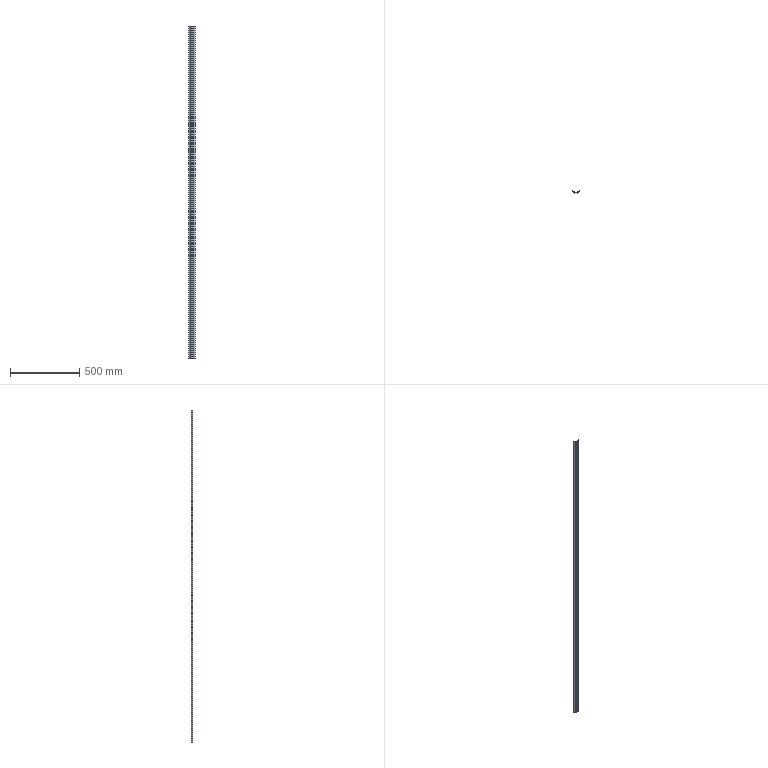Part | SolidWorks | features Extrusion 1 | 1 solid | 32 faces | box 46.782 x 13.535 x 2390 mm | volume 191944 mm3 | plane 25 | cylinder 7 | commonest cylinder face diameters 67.994 x4 0.2 x2 65.594 x1
STEP:
#1=CARTESIAN_POINT('',(-11.25,9.786,-1195.));
#2=VERTEX_POINT('',#1);
#3=CARTESIAN_POINT('',(-11.25,5.783,-1195.));
#4=VERTEX_POINT('',#3);
#5=CARTESIAN_POINT('',(-11.25,9.786,-1195.));
#6=DIRECTION('',(0.,-1.,0.));
#7=VECTOR('',#6,1000.);
#8=LINE('',#5,#7);
#9=EDGE_CURVE('',#2,#4,#8,.T.);
#10=ORIENTED_EDGE('',*,*,#9,.T.);
#11=CARTESIAN_POINT('',(-11.25,5.783,1195.));
#12=VERTEX_POINT('',#11);
#13=CARTESIAN_POINT('',(-11.25,5.783,1195.));
#14=DIRECTION('',(0.,0.,-1.));
#15=VECTOR('',#14,1000.);
#16=LINE('',#13,#15);
#17=EDGE_CURVE('',#12,#4,#16,.T.);
#18=ORIENTED_EDGE('',*,*,#17,.F.);
#19=CARTESIAN_POINT('',(-11.25,9.786,1195.));
#20=VERTEX_POINT('',#19);
#21=CARTESIAN_POINT('',(-11.25,9.786,1195.));
#22=DIRECTION('',(0.,-1.,0.));
#23=VECTOR('',#22,1000.);
#24=LINE('',#21,#23);
#25=EDGE_CURVE('',#20,#12,#24,.T.);
#26=ORIENTED_EDGE('',*,*,#25,.F.);
#27=CARTESIAN_POINT('',(-11.25,9.786,1195.));
#28=DIRECTION('',(0.,0.,-1.));
#29=VECTOR('',#28,1000.);
#30=LINE('',#27,#29);
#31=EDGE_CURVE('',#20,#2,#30,.T.);
#32=ORIENTED_EDGE('',*,*,#31,.T.);
#33=EDGE_LOOP('',(#10,#18,#26,#32));
#34=FACE_OUTER_BOUND('',#33,.T.);
#35=CARTESIAN_POINT('',(-11.25,9.786,1195.));
#36=DIRECTION('',(1.,0.,0.));
#37=DIRECTION('',(0.,0.,-1.));
#38=AXIS2_PLACEMENT_3D('',#35,#36,#37);
#39=PLANE('',#38);
#40=ADVANCED_FACE('',(#34),#39,.F.);
#41=CARTESIAN_POINT('',(-10.667,5.2,-1195.));
#42=VERTEX_POINT('',#41);
#43=CARTESIAN_POINT('',(-11.25,5.783,-1195.));
#44=DIRECTION('',(0.7071,-0.7071,0.));
#45=VECTOR('',#44,1000.);
#46=LINE('',#43,#45);
#47=EDGE_CURVE('',#4,#42,#46,.T.);
#48=ORIENTED_EDGE('',*,*,#47,.T.);
#49=CARTESIAN_POINT('',(-10.667,5.2,1195.));
#50=VERTEX_POINT('',#49);
#51=CARTESIAN_POINT('',(-10.667,5.2,1195.));
#52=DIRECTION('',(0.,0.,-1.));
#53=VECTOR('',#52,1000.);
#54=LINE('',#51,#53);
#55=EDGE_CURVE('',#50,#42,#54,.T.);
#56=ORIENTED_EDGE('',*,*,#55,.F.);
#57=CARTESIAN_POINT('',(-11.25,5.783,1195.));
#58=DIRECTION('',(0.7071,-0.7071,0.));
#59=VECTOR('',#58,1000.);
#60=LINE('',#57,#59);
#61=EDGE_CURVE('',#12,#50,#60,.T.);
#62=ORIENTED_EDGE('',*,*,#61,.F.);
#63=ORIENTED_EDGE('',*,*,#17,.T.);
#64=EDGE_LOOP('',(#48,#56,#62,#63));
#65=FACE_OUTER_BOUND('',#64,.T.);
#66=CARTESIAN_POINT('',(-11.25,5.783,1195.));
#67=DIRECTION('',(0.7071,0.7071,0.));
#68=DIRECTION('',(-0.7071,0.7071,0.));
#69=AXIS2_PLACEMENT_3D('',#66,#67,#68);
#70=PLANE('',#69);
#71=ADVANCED_FACE('',(#65),#70,.F.);
#72=CARTESIAN_POINT('',(-8.25,5.2,-1195.));
#73=VERTEX_POINT('',#72);
#74=CARTESIAN_POINT('',(-10.667,5.2,-1195.));
#75=DIRECTION('',(1.,0.,0.));
#76=VECTOR('',#75,1000.);
#77=LINE('',#74,#76);
#78=EDGE_CURVE('',#42,#73,#77,.T.);
#79=ORIENTED_EDGE('',*,*,#78,.T.);
#80=CARTESIAN_POINT('',(-8.25,5.2,1195.));
#81=VERTEX_POINT('',#80);
#82=CARTESIAN_POINT('',(-8.25,5.2,1195.));
#83=DIRECTION('',(0.,0.,-1.));
#84=VECTOR('',#83,1000.);
#85=LINE('',#82,#84);
#86=EDGE_CURVE('',#81,#73,#85,.T.);
#87=ORIENTED_EDGE('',*,*,#86,.F.);
#88=CARTESIAN_POINT('',(-10.667,5.2,1195.));
#89=DIRECTION('',(1.,0.,0.));
#90=VECTOR('',#89,1000.);
#91=LINE('',#88,#90);
#92=EDGE_CURVE('',#50,#81,#91,.T.);
#93=ORIENTED_EDGE('',*,*,#92,.F.);
#94=ORIENTED_EDGE('',*,*,#55,.T.);
#95=EDGE_LOOP('',(#79,#87,#93,#94));
#96=FACE_OUTER_BOUND('',#95,.T.);
#97=CARTESIAN_POINT('',(-10.667,5.2,1195.));
#98=DIRECTION('',(0.,1.,0.));
#99=DIRECTION('',(0.,0.,1.));
#100=AXIS2_PLACEMENT_3D('',#97,#98,#99);
#101=PLANE('',#100);
#102=ADVANCED_FACE('',(#96),#101,.F.);
#103=CARTESIAN_POINT('',(-8.25,6.,-1195.));
#104=VERTEX_POINT('',#103);
#105=CARTESIAN_POINT('',(-8.25,5.2,-1195.));
#106=DIRECTION('',(0.,1.,0.));
#107=VECTOR('',#106,1000.);
#108=LINE('',#105,#107);
#109=EDGE_CURVE('',#73,#104,#108,.T.);
#110=ORIENTED_EDGE('',*,*,#109,.T.);
#111=CARTESIAN_POINT('',(-8.25,6.,1195.));
#112=VERTEX_POINT('',#111);
#113=CARTESIAN_POINT('',(-8.25,6.,1195.));
#114=DIRECTION('',(0.,0.,-1.));
#115=VECTOR('',#114,1000.);
#116=LINE('',#113,#115);
#117=EDGE_CURVE('',#112,#104,#116,.T.);
#118=ORIENTED_EDGE('',*,*,#117,.F.);
#119=CARTESIAN_POINT('',(-8.25,5.2,1195.));
#120=DIRECTION('',(0.,1.,0.));
#121=VECTOR('',#120,1000.);
#122=LINE('',#119,#121);
#123=EDGE_CURVE('',#81,#112,#122,.T.);
#124=ORIENTED_EDGE('',*,*,#123,.F.);
#125=ORIENTED_EDGE('',*,*,#86,.T.);
#126=EDGE_LOOP('',(#110,#118,#124,#125));
#127=FACE_OUTER_BOUND('',#126,.T.);
#128=CARTESIAN_POINT('',(-8.25,5.2,1195.));
#129=DIRECTION('',(-1.,0.,0.));
#130=DIRECTION('',(0.,0.,1.));
#131=AXIS2_PLACEMENT_3D('',#128,#129,#130);
#132=PLANE('',#131);
#133=ADVANCED_FACE('',(#127),#132,.F.);
#134=CARTESIAN_POINT('',(-10.25,6.,-1195.));
#135=VERTEX_POINT('',#134);
#136=CARTESIAN_POINT('',(-8.25,6.,-1195.));
#137=DIRECTION('',(-1.,0.,0.));
#138=VECTOR('',#137,1000.);
#139=LINE('',#136,#138);
#140=EDGE_CURVE('',#104,#135,#139,.T.);
#141=ORIENTED_EDGE('',*,*,#140,.T.);
#142=CARTESIAN_POINT('',(-10.25,6.,1195.));
#143=VERTEX_POINT('',#142);
#144=CARTESIAN_POINT('',(-10.25,6.,1195.));
#145=DIRECTION('',(0.,0.,-1.));
#146=VECTOR('',#145,1000.);
#147=LINE('',#144,#146);
#148=EDGE_CURVE('',#143,#135,#147,.T.);
#149=ORIENTED_EDGE('',*,*,#148,.F.);
#150=CARTESIAN_POINT('',(-8.25,6.,1195.));
#151=DIRECTION('',(-1.,0.,0.));
#152=VECTOR('',#151,1000.);
#153=LINE('',#150,#152);
#154=EDGE_CURVE('',#112,#143,#153,.T.);
#155=ORIENTED_EDGE('',*,*,#154,.F.);
#156=ORIENTED_EDGE('',*,*,#117,.T.);
#157=EDGE_LOOP('',(#141,#149,#155,#156));
#158=FACE_OUTER_BOUND('',#157,.T.);
#159=CARTESIAN_POINT('',(-8.25,6.,1195.));
#160=DIRECTION('',(0.,-1.,0.));
#161=DIRECTION('',(0.,0.,-1.));
#162=AXIS2_PLACEMENT_3D('',#159,#160,#161);
#163=PLANE('',#162);
#164=ADVANCED_FACE('',(#158),#163,.F.);
#165=CARTESIAN_POINT('',(-10.25,7.726,-1195.));
#166=VERTEX_POINT('',#165);
#167=CARTESIAN_POINT('',(-10.25,6.,-1195.));
#168=DIRECTION('',(0.,1.,0.));
#169=VECTOR('',#168,1000.);
#170=LINE('',#167,#169);
#171=EDGE_CURVE('',#135,#166,#170,.T.);
#172=ORIENTED_EDGE('',*,*,#171,.T.);
#173=CARTESIAN_POINT('',(-10.25,7.726,1195.));
#174=VERTEX_POINT('',#173);
#175=CARTESIAN_POINT('',(-10.25,7.726,1195.));
#176=DIRECTION('',(0.,0.,-1.));
#177=VECTOR('',#176,1000.);
#178=LINE('',#175,#177);
#179=EDGE_CURVE('',#174,#166,#178,.T.);
#180=ORIENTED_EDGE('',*,*,#179,.F.);
#181=CARTESIAN_POINT('',(-10.25,6.,1195.));
#182=DIRECTION('',(0.,1.,0.));
#183=VECTOR('',#182,1000.);
#184=LINE('',#181,#183);
#185=EDGE_CURVE('',#143,#174,#184,.T.);
#186=ORIENTED_EDGE('',*,*,#185,.F.);
#187=ORIENTED_EDGE('',*,*,#148,.T.);
#188=EDGE_LOOP('',(#172,#180,#186,#187));
#189=FACE_OUTER_BOUND('',#188,.T.);
#190=CARTESIAN_POINT('',(-10.25,6.,1195.));
#191=DIRECTION('',(-1.,0.,0.));
#192=DIRECTION('',(0.,0.,1.));
#193=AXIS2_PLACEMENT_3D('',#190,#191,#192);
#194=PLANE('',#193);
#195=ADVANCED_FACE('',(#189),#194,.F.);
#196=CARTESIAN_POINT('',(-9.,7.725,-1195.));
#197=VERTEX_POINT('',#196);
#198=CARTESIAN_POINT('',(-10.25,7.726,-1195.));
#199=DIRECTION('',(1.,-0.001291,0.));
#200=VECTOR('',#199,1000.);
#201=LINE('',#198,#200);
#202=EDGE_CURVE('',#166,#197,#201,.T.);
#203=ORIENTED_EDGE('',*,*,#202,.T.);
#204=CARTESIAN_POINT('',(-9.,7.725,1195.));
#205=VERTEX_POINT('',#204);
#206=CARTESIAN_POINT('',(-9.,7.725,1195.));
#207=DIRECTION('',(0.,0.,-1.));
#208=VECTOR('',#207,1000.);
#209=LINE('',#206,#208);
#210=EDGE_CURVE('',#205,#197,#209,.T.);
#211=ORIENTED_EDGE('',*,*,#210,.F.);
#212=CARTESIAN_POINT('',(-10.25,7.726,1195.));
#213=DIRECTION('',(1.,-0.001291,0.));
#214=VECTOR('',#213,1000.);
#215=LINE('',#212,#214);
#216=EDGE_CURVE('',#174,#205,#215,.T.);
#217=ORIENTED_EDGE('',*,*,#216,.F.);
#218=ORIENTED_EDGE('',*,*,#179,.T.);
#219=EDGE_LOOP('',(#203,#211,#217,#218));
#220=FACE_OUTER_BOUND('',#219,.T.);
#221=CARTESIAN_POINT('',(-10.25,7.726,1195.));
#222=DIRECTION('',(0.001291,1.,0.));
#223=DIRECTION('',(-1.,0.001291,0.));
#224=AXIS2_PLACEMENT_3D('',#221,#222,#223);
#225=PLANE('',#224);
#226=ADVANCED_FACE('',(#220),#225,.F.);
#227=CARTESIAN_POINT('',(-8.25,8.474,-1195.));
#228=VERTEX_POINT('',#227);
#229=CARTESIAN_POINT('',(-9.,7.725,-1195.));
#230=DIRECTION('',(0.7076,0.7067,0.));
#231=VECTOR('',#230,1000.);
#232=LINE('',#229,#231);
#233=EDGE_CURVE('',#197,#228,#232,.T.);
#234=ORIENTED_EDGE('',*,*,#233,.T.);
#235=CARTESIAN_POINT('',(-8.25,8.474,1195.));
#236=VERTEX_POINT('',#235);
#237=CARTESIAN_POINT('',(-8.25,8.474,1195.));
#238=DIRECTION('',(0.,0.,-1.));
#239=VECTOR('',#238,1000.);
#240=LINE('',#237,#239);
#241=EDGE_CURVE('',#236,#228,#240,.T.);
#242=ORIENTED_EDGE('',*,*,#241,.F.);
#243=CARTESIAN_POINT('',(-9.,7.725,1195.));
#244=DIRECTION('',(0.7076,0.7067,0.));
#245=VECTOR('',#244,1000.);
#246=LINE('',#243,#245);
#247=EDGE_CURVE('',#205,#236,#246,.T.);
#248=ORIENTED_EDGE('',*,*,#247,.F.);
#249=ORIENTED_EDGE('',*,*,#210,.T.);
#250=EDGE_LOOP('',(#234,#242,#248,#249));
#251=FACE_OUTER_BOUND('',#250,.T.);
#252=CARTESIAN_POINT('',(-9.,7.725,1195.));
#253=DIRECTION('',(-0.7067,0.7076,0.));
#254=DIRECTION('',(-0.7076,-0.7067,0.));
#255=AXIS2_PLACEMENT_3D('',#252,#253,#254);
#256=PLANE('',#255);
#257=ADVANCED_FACE('',(#251),#256,.F.);
#258=CARTESIAN_POINT('',(-8.25,8.887,-1195.));
#259=VERTEX_POINT('',#258);
#260=CARTESIAN_POINT('',(-8.25,8.474,-1195.));
#261=DIRECTION('',(0.,1.,0.));
#262=VECTOR('',#261,1000.);
#263=LINE('',#260,#262);
#264=EDGE_CURVE('',#228,#259,#263,.T.);
#265=ORIENTED_EDGE('',*,*,#264,.T.);
#266=CARTESIAN_POINT('',(-8.25,8.887,1195.));
#267=VERTEX_POINT('',#266);
#268=CARTESIAN_POINT('',(-8.25,8.887,1195.));
#269=DIRECTION('',(0.,0.,-1.));
#270=VECTOR('',#269,1000.);
#271=LINE('',#268,#270);
#272=EDGE_CURVE('',#267,#259,#271,.T.);
#273=ORIENTED_EDGE('',*,*,#272,.F.);
#274=CARTESIAN_POINT('',(-8.25,8.474,1195.));
#275=DIRECTION('',(0.,1.,0.));
#276=VECTOR('',#275,1000.);
#277=LINE('',#274,#276);
#278=EDGE_CURVE('',#236,#267,#277,.T.);
#279=ORIENTED_EDGE('',*,*,#278,.F.);
#280=ORIENTED_EDGE('',*,*,#241,.T.);
#281=EDGE_LOOP('',(#265,#273,#279,#280));
#282=FACE_OUTER_BOUND('',#281,.T.);
#283=CARTESIAN_POINT('',(-8.25,8.474,1195.));
#284=DIRECTION('',(-1.,0.,0.));
#285=DIRECTION('',(0.,0.,1.));
#286=AXIS2_PLACEMENT_3D('',#283,#284,#285);
#287=PLANE('',#286);
#288=ADVANCED_FACE('',(#282),#287,.F.);
#289=CARTESIAN_POINT('',(-3.,8.003,-1195.));
#290=VERTEX_POINT('',#289);
#291=CARTESIAN_POINT('',(0.,41.867,-1195.));
#292=DIRECTION('',(0.,0.,1.));
#293=DIRECTION('',(1.,0.,0.));
#294=AXIS2_PLACEMENT_3D('',#291,#292,#293);
#295=CIRCLE('',#294,33.997);
#296=EDGE_CURVE('',#259,#290,#295,.T.);
#297=ORIENTED_EDGE('',*,*,#296,.T.);
#298=CARTESIAN_POINT('',(-3.,8.003,1195.));
#299=VERTEX_POINT('',#298);
#300=CARTESIAN_POINT('',(-3.,8.003,1195.));
#301=DIRECTION('',(0.,0.,-1.));
#302=VECTOR('',#301,1000.);
#303=LINE('',#300,#302);
#304=EDGE_CURVE('',#299,#290,#303,.T.);
#305=ORIENTED_EDGE('',*,*,#304,.F.);
#306=CARTESIAN_POINT('',(0.,41.867,1195.));
#307=DIRECTION('',(0.,0.,1.));
#308=DIRECTION('',(1.,0.,0.));
#309=AXIS2_PLACEMENT_3D('',#306,#307,#308);
#310=CIRCLE('',#309,33.997);
#311=EDGE_CURVE('',#267,#299,#310,.T.);
#312=ORIENTED_EDGE('',*,*,#311,.F.);
#313=ORIENTED_EDGE('',*,*,#272,.T.);
#314=EDGE_LOOP('',(#297,#305,#312,#313));
#315=FACE_OUTER_BOUND('',#314,.T.);
#316=CARTESIAN_POINT('',(0.,41.867,1195.));
#317=DIRECTION('',(0.,0.,-1.));
#318=DIRECTION('',(-1.,0.,0.));
#319=AXIS2_PLACEMENT_3D('',#316,#317,#318);
#320=CYLINDRICAL_SURFACE('',#319,33.997);
#321=ADVANCED_FACE('',(#315),#320,.T.);
#322=CARTESIAN_POINT('',(-3.,7.702,-1195.));
#323=VERTEX_POINT('',#322);
#324=CARTESIAN_POINT('',(-3.,8.003,-1195.));
#325=DIRECTION('',(0.,-1.,0.));
#326=VECTOR('',#325,1000.);
#327=LINE('',#324,#326);
#328=EDGE_CURVE('',#290,#323,#327,.T.);
#329=ORIENTED_EDGE('',*,*,#328,.T.);
#330=CARTESIAN_POINT('',(-3.,7.702,1195.));
#331=VERTEX_POINT('',#330);
#332=CARTESIAN_POINT('',(-3.,7.702,1195.));
#333=DIRECTION('',(0.,0.,-1.));
#334=VECTOR('',#333,1000.);
#335=LINE('',#332,#334);
#336=EDGE_CURVE('',#331,#323,#335,.T.);
#337=ORIENTED_EDGE('',*,*,#336,.F.);
#338=CARTESIAN_POINT('',(-3.,8.003,1195.));
#339=DIRECTION('',(0.,-1.,0.));
#340=VECTOR('',#339,1000.);
#341=LINE('',#338,#340);
#342=EDGE_CURVE('',#299,#331,#341,.T.);
#343=ORIENTED_EDGE('',*,*,#342,.F.);
#344=ORIENTED_EDGE('',*,*,#304,.T.);
#345=EDGE_LOOP('',(#329,#337,#343,#344));
#346=FACE_OUTER_BOUND('',#345,.T.);
#347=CARTESIAN_POINT('',(-3.,8.003,1195.));
#348=DIRECTION('',(1.,0.,0.));
#349=DIRECTION('',(0.,0.,-1.));
#350=AXIS2_PLACEMENT_3D('',#347,#348,#349);
#351=PLANE('',#350);
#352=ADVANCED_FACE('',(#346),#351,.F.);
#353=CARTESIAN_POINT('',(3.,7.702,-1195.));
#354=VERTEX_POINT('',#353);
#355=CARTESIAN_POINT('',(-3.,7.702,-1195.));
#356=DIRECTION('',(1.,0.,0.));
#357=VECTOR('',#356,1000.);
#358=LINE('',#355,#357);
#359=EDGE_CURVE('',#323,#354,#358,.T.);
#360=ORIENTED_EDGE('',*,*,#359,.T.);
#361=CARTESIAN_POINT('',(3.,7.702,1195.));
#362=VERTEX_POINT('',#361);
#363=CARTESIAN_POINT('',(3.,7.702,1195.));
#364=DIRECTION('',(0.,0.,-1.));
#365=VECTOR('',#364,1000.);
#366=LINE('',#363,#365);
#367=EDGE_CURVE('',#362,#354,#366,.T.);
#368=ORIENTED_EDGE('',*,*,#367,.F.);
#369=CARTESIAN_POINT('',(-3.,7.702,1195.));
#370=DIRECTION('',(1.,0.,0.));
#371=VECTOR('',#370,1000.);
#372=LINE('',#369,#371);
#373=EDGE_CURVE('',#331,#362,#372,.T.);
#374=ORIENTED_EDGE('',*,*,#373,.F.);
#375=ORIENTED_EDGE('',*,*,#336,.T.);
#376=EDGE_LOOP('',(#360,#368,#374,#375));
#377=FACE_OUTER_BOUND('',#376,.T.);
#378=CARTESIAN_POINT('',(-3.,7.702,1195.));
#379=DIRECTION('',(0.,1.,0.));
#380=DIRECTION('',(0.,0.,1.));
#381=AXIS2_PLACEMENT_3D('',#378,#379,#380);
#382=PLANE('',#381);
#383=ADVANCED_FACE('',(#377),#382,.F.);
#384=CARTESIAN_POINT('',(3.,8.003,-1195.));
#385=VERTEX_POINT('',#384);
#386=CARTESIAN_POINT('',(3.,7.702,-1195.));
#387=DIRECTION('',(0.,1.,0.));
#388=VECTOR('',#387,1000.);
#389=LINE('',#386,#388);
#390=EDGE_CURVE('',#354,#385,#389,.T.);
#391=ORIENTED_EDGE('',*,*,#390,.T.);
#392=CARTESIAN_POINT('',(3.,8.003,1195.));
#393=VERTEX_POINT('',#392);
#394=CARTESIAN_POINT('',(3.,8.003,1195.));
#395=DIRECTION('',(0.,0.,-1.));
#396=VECTOR('',#395,1000.);
#397=LINE('',#394,#396);
#398=EDGE_CURVE('',#393,#385,#397,.T.);
#399=ORIENTED_EDGE('',*,*,#398,.F.);
#400=CARTESIAN_POINT('',(3.,7.702,1195.));
#401=DIRECTION('',(0.,1.,0.));
#402=VECTOR('',#401,1000.);
#403=LINE('',#400,#402);
#404=EDGE_CURVE('',#362,#393,#403,.T.);
#405=ORIENTED_EDGE('',*,*,#404,.F.);
#406=ORIENTED_EDGE('',*,*,#367,.T.);
#407=EDGE_LOOP('',(#391,#399,#405,#406));
#408=FACE_OUTER_BOUND('',#407,.T.);
#409=CARTESIAN_POINT('',(3.,7.702,1195.));
#410=DIRECTION('',(-1.,0.,0.));
#411=DIRECTION('',(0.,0.,1.));
#412=AXIS2_PLACEMENT_3D('',#409,#410,#411);
#413=PLANE('',#412);
#414=ADVANCED_FACE('',(#408),#413,.F.);
#415=CARTESIAN_POINT('',(8.25,8.887,-1195.));
#416=VERTEX_POINT('',#415);
#417=CARTESIAN_POINT('',(0.,41.867,-1195.));
#418=DIRECTION('',(0.,0.,1.));
#419=DIRECTION('',(1.,0.,0.));
#420=AXIS2_PLACEMENT_3D('',#417,#418,#419);
#421=CIRCLE('',#420,33.997);
#422=EDGE_CURVE('',#385,#416,#421,.T.);
#423=ORIENTED_EDGE('',*,*,#422,.T.);
#424=CARTESIAN_POINT('',(8.25,8.887,1195.));
#425=VERTEX_POINT('',#424);
#426=CARTESIAN_POINT('',(8.25,8.887,1195.));
#427=DIRECTION('',(0.,0.,-1.));
#428=VECTOR('',#427,1000.);
#429=LINE('',#426,#428);
#430=EDGE_CURVE('',#425,#416,#429,.T.);
#431=ORIENTED_EDGE('',*,*,#430,.F.);
#432=CARTESIAN_POINT('',(0.,41.867,1195.));
#433=DIRECTION('',(0.,0.,1.));
#434=DIRECTION('',(1.,0.,0.));
#435=AXIS2_PLACEMENT_3D('',#432,#433,#434);
#436=CIRCLE('',#435,33.997);
#437=EDGE_CURVE('',#393,#425,#436,.T.);
#438=ORIENTED_EDGE('',*,*,#437,.F.);
#439=ORIENTED_EDGE('',*,*,#398,.T.);
#440=EDGE_LOOP('',(#423,#431,#438,#439));
#441=FACE_OUTER_BOUND('',#440,.T.);
#442=CARTESIAN_POINT('',(0.,41.867,1195.));
#443=DIRECTION('',(0.,0.,-1.));
#444=DIRECTION('',(-1.,0.,0.));
#445=AXIS2_PLACEMENT_3D('',#442,#443,#444);
#446=CYLINDRICAL_SURFACE('',#445,33.997);
#447=ADVANCED_FACE('',(#441),#446,.T.);
#448=CARTESIAN_POINT('',(8.25,8.474,-1195.));
#449=VERTEX_POINT('',#448);
#450=CARTESIAN_POINT('',(8.25,8.887,-1195.));
#451=DIRECTION('',(0.,-1.,0.));
#452=VECTOR('',#451,1000.);
#453=LINE('',#450,#452);
#454=EDGE_CURVE('',#416,#449,#453,.T.);
#455=ORIENTED_EDGE('',*,*,#454,.T.);
#456=CARTESIAN_POINT('',(8.25,8.474,1195.));
#457=VERTEX_POINT('',#456);
#458=CARTESIAN_POINT('',(8.25,8.474,1195.));
#459=DIRECTION('',(0.,0.,-1.));
#460=VECTOR('',#459,1000.);
#461=LINE('',#458,#460);
#462=EDGE_CURVE('',#457,#449,#461,.T.);
#463=ORIENTED_EDGE('',*,*,#462,.F.);
#464=CARTESIAN_POINT('',(8.25,8.887,1195.));
#465=DIRECTION('',(0.,-1.,0.));
#466=VECTOR('',#465,1000.);
#467=LINE('',#464,#466);
#468=EDGE_CURVE('',#425,#457,#467,.T.);
#469=ORIENTED_EDGE('',*,*,#468,.F.);
#470=ORIENTED_EDGE('',*,*,#430,.T.);
#471=EDGE_LOOP('',(#455,#463,#469,#470));
#472=FACE_OUTER_BOUND('',#471,.T.);
#473=CARTESIAN_POINT('',(8.25,8.887,1195.));
#474=DIRECTION('',(1.,0.,0.));
#475=DIRECTION('',(0.,0.,-1.));
#476=AXIS2_PLACEMENT_3D('',#473,#474,#475);
#477=PLANE('',#476);
#478=ADVANCED_FACE('',(#472),#477,.F.);
#479=CARTESIAN_POINT('',(9.,7.725,-1195.));
#480=VERTEX_POINT('',#479);
#481=CARTESIAN_POINT('',(8.25,8.474,-1195.));
#482=DIRECTION('',(0.7076,-0.7067,0.));
#483=VECTOR('',#482,1000.);
#484=LINE('',#481,#483);
#485=EDGE_CURVE('',#449,#480,#484,.T.);
#486=ORIENTED_EDGE('',*,*,#485,.T.);
#487=CARTESIAN_POINT('',(9.,7.725,1195.));
#488=VERTEX_POINT('',#487);
#489=CARTESIAN_POINT('',(9.,7.725,1195.));
#490=DIRECTION('',(0.,0.,-1.));
#491=VECTOR('',#490,1000.);
#492=LINE('',#489,#491);
#493=EDGE_CURVE('',#488,#480,#492,.T.);
#494=ORIENTED_EDGE('',*,*,#493,.F.);
#495=CARTESIAN_POINT('',(8.25,8.474,1195.));
#496=DIRECTION('',(0.7076,-0.7067,0.));
#497=VECTOR('',#496,1000.);
#498=LINE('',#495,#497);
#499=EDGE_CURVE('',#457,#488,#498,.T.);
#500=ORIENTED_EDGE('',*,*,#499,.F.);
#501=ORIENTED_EDGE('',*,*,#462,.T.);
#502=EDGE_LOOP('',(#486,#494,#500,#501));
#503=FACE_OUTER_BOUND('',#502,.T.);
#504=CARTESIAN_POINT('',(8.25,8.474,1195.));
#505=DIRECTION('',(0.7067,0.7076,0.));
#506=DIRECTION('',(-0.7076,0.7067,0.));
#507=AXIS2_PLACEMENT_3D('',#504,#505,#506);
#508=PLANE('',#507);
#509=ADVANCED_FACE('',(#503),#508,.F.);
#510=CARTESIAN_POINT('',(10.25,7.726,-1195.));
#511=VERTEX_POINT('',#510);
#512=CARTESIAN_POINT('',(9.,7.725,-1195.));
#513=DIRECTION('',(1.,0.001291,0.));
#514=VECTOR('',#513,1000.);
#515=LINE('',#512,#514);
#516=EDGE_CURVE('',#480,#511,#515,.T.);
#517=ORIENTED_EDGE('',*,*,#516,.T.);
#518=CARTESIAN_POINT('',(10.25,7.726,1195.));
#519=VERTEX_POINT('',#518);
#520=CARTESIAN_POINT('',(10.25,7.726,1195.));
#521=DIRECTION('',(0.,0.,-1.));
#522=VECTOR('',#521,1000.);
#523=LINE('',#520,#522);
#524=EDGE_CURVE('',#519,#511,#523,.T.);
#525=ORIENTED_EDGE('',*,*,#524,.F.);
#526=CARTESIAN_POINT('',(9.,7.725,1195.));
#527=DIRECTION('',(1.,0.001291,0.));
#528=VECTOR('',#527,1000.);
#529=LINE('',#526,#528);
#530=EDGE_CURVE('',#488,#519,#529,.T.);
#531=ORIENTED_EDGE('',*,*,#530,.F.);
#532=ORIENTED_EDGE('',*,*,#493,.T.);
#533=EDGE_LOOP('',(#517,#525,#531,#532));
#534=FACE_OUTER_BOUND('',#533,.T.);
#535=CARTESIAN_POINT('',(9.,7.725,1195.));
#536=DIRECTION('',(-0.001291,1.,0.));
#537=DIRECTION('',(-1.,-0.001291,0.));
#538=AXIS2_PLACEMENT_3D('',#535,#536,#537);
#539=PLANE('',#538);
#540=ADVANCED_FACE('',(#534),#539,.F.);
#541=CARTESIAN_POINT('',(10.25,6.,-1195.));
#542=VERTEX_POINT('',#541);
#543=CARTESIAN_POINT('',(10.25,7.726,-1195.));
#544=DIRECTION('',(0.,-1.,0.));
#545=VECTOR('',#544,1000.);
#546=LINE('',#543,#545);
#547=EDGE_CURVE('',#511,#542,#546,.T.);
#548=ORIENTED_EDGE('',*,*,#547,.T.);
#549=CARTESIAN_POINT('',(10.25,6.,1195.));
#550=VERTEX_POINT('',#549);
#551=CARTESIAN_POINT('',(10.25,6.,1195.));
#552=DIRECTION('',(0.,0.,-1.));
#553=VECTOR('',#552,1000.);
#554=LINE('',#551,#553);
#555=EDGE_CURVE('',#550,#542,#554,.T.);
#556=ORIENTED_EDGE('',*,*,#555,.F.);
#557=CARTESIAN_POINT('',(10.25,7.726,1195.));
#558=DIRECTION('',(0.,-1.,0.));
#559=VECTOR('',#558,1000.);
#560=LINE('',#557,#559);
#561=EDGE_CURVE('',#519,#550,#560,.T.);
#562=ORIENTED_EDGE('',*,*,#561,.F.);
#563=ORIENTED_EDGE('',*,*,#524,.T.);
#564=EDGE_LOOP('',(#548,#556,#562,#563));
#565=FACE_OUTER_BOUND('',#564,.T.);
#566=CARTESIAN_POINT('',(10.25,7.726,1195.));
#567=DIRECTION('',(1.,0.,0.));
#568=DIRECTION('',(0.,0.,-1.));
#569=AXIS2_PLACEMENT_3D('',#566,#567,#568);
#570=PLANE('',#569);
#571=ADVANCED_FACE('',(#565),#570,.F.);
#572=CARTESIAN_POINT('',(8.25,6.,-1195.));
#573=VERTEX_POINT('',#572);
#574=CARTESIAN_POINT('',(10.25,6.,-1195.));
#575=DIRECTION('',(-1.,0.,0.));
#576=VECTOR('',#575,1000.);
#577=LINE('',#574,#576);
#578=EDGE_CURVE('',#542,#573,#577,.T.);
#579=ORIENTED_EDGE('',*,*,#578,.T.);
#580=CARTESIAN_POINT('',(8.25,6.,1195.));
#581=VERTEX_POINT('',#580);
#582=CARTESIAN_POINT('',(8.25,6.,1195.));
#583=DIRECTION('',(0.,0.,-1.));
#584=VECTOR('',#583,1000.);
#585=LINE('',#582,#584);
#586=EDGE_CURVE('',#581,#573,#585,.T.);
#587=ORIENTED_EDGE('',*,*,#586,.F.);
#588=CARTESIAN_POINT('',(10.25,6.,1195.));
#589=DIRECTION('',(-1.,0.,0.));
#590=VECTOR('',#589,1000.);
#591=LINE('',#588,#590);
#592=EDGE_CURVE('',#550,#581,#591,.T.);
#593=ORIENTED_EDGE('',*,*,#592,.F.);
#594=ORIENTED_EDGE('',*,*,#555,.T.);
#595=EDGE_LOOP('',(#579,#587,#593,#594));
#596=FACE_OUTER_BOUND('',#595,.T.);
#597=CARTESIAN_POINT('',(10.25,6.,1195.));
#598=DIRECTION('',(0.,-1.,0.));
#599=DIRECTION('',(0.,0.,-1.));
#600=AXIS2_PLACEMENT_3D('',#597,#598,#599);
#601=PLANE('',#600);
#602=ADVANCED_FACE('',(#596),#601,.F.);
#603=CARTESIAN_POINT('',(8.25,5.2,-1195.));
#604=VERTEX_POINT('',#603);
#605=CARTESIAN_POINT('',(8.25,6.,-1195.));
#606=DIRECTION('',(0.,-1.,0.));
#607=VECTOR('',#606,1000.);
#608=LINE('',#605,#607);
#609=EDGE_CURVE('',#573,#604,#608,.T.);
#610=ORIENTED_EDGE('',*,*,#609,.T.);
#611=CARTESIAN_POINT('',(8.25,5.2,1195.));
#612=VERTEX_POINT('',#611);
#613=CARTESIAN_POINT('',(8.25,5.2,1195.));
#614=DIRECTION('',(0.,0.,-1.));
#615=VECTOR('',#614,1000.);
#616=LINE('',#613,#615);
#617=EDGE_CURVE('',#612,#604,#616,.T.);
#618=ORIENTED_EDGE('',*,*,#617,.F.);
#619=CARTESIAN_POINT('',(8.25,6.,1195.));
#620=DIRECTION('',(0.,-1.,0.));
#621=VECTOR('',#620,1000.);
#622=LINE('',#619,#621);
#623=EDGE_CURVE('',#581,#612,#622,.T.);
#624=ORIENTED_EDGE('',*,*,#623,.F.);
#625=ORIENTED_EDGE('',*,*,#586,.T.);
#626=EDGE_LOOP('',(#610,#618,#624,#625));
#627=FACE_OUTER_BOUND('',#626,.T.);
#628=CARTESIAN_POINT('',(8.25,6.,1195.));
#629=DIRECTION('',(1.,0.,0.));
#630=DIRECTION('',(0.,0.,-1.));
#631=AXIS2_PLACEMENT_3D('',#628,#629,#630);
#632=PLANE('',#631);
#633=ADVANCED_FACE('',(#627),#632,.F.);
#634=CARTESIAN_POINT('',(10.667,5.2,-1195.));
#635=VERTEX_POINT('',#634);
#636=CARTESIAN_POINT('',(8.25,5.2,-1195.));
#637=DIRECTION('',(1.,0.,0.));
#638=VECTOR('',#637,1000.);
#639=LINE('',#636,#638);
#640=EDGE_CURVE('',#604,#635,#639,.T.);
#641=ORIENTED_EDGE('',*,*,#640,.T.);
#642=CARTESIAN_POINT('',(10.667,5.2,1195.));
#643=VERTEX_POINT('',#642);
#644=CARTESIAN_POINT('',(10.667,5.2,1195.));
#645=DIRECTION('',(0.,0.,-1.));
#646=VECTOR('',#645,1000.);
#647=LINE('',#644,#646);
#648=EDGE_CURVE('',#643,#635,#647,.T.);
#649=ORIENTED_EDGE('',*,*,#648,.F.);
#650=CARTESIAN_POINT('',(8.25,5.2,1195.));
#651=DIRECTION('',(1.,0.,0.));
#652=VECTOR('',#651,1000.);
#653=LINE('',#650,#652);
#654=EDGE_CURVE('',#612,#643,#653,.T.);
#655=ORIENTED_EDGE('',*,*,#654,.F.);
#656=ORIENTED_EDGE('',*,*,#617,.T.);
#657=EDGE_LOOP('',(#641,#649,#655,#656));
#658=FACE_OUTER_BOUND('',#657,.T.);
#659=CARTESIAN_POINT('',(8.25,5.2,1195.));
#660=DIRECTION('',(0.,1.,0.));
#661=DIRECTION('',(0.,0.,1.));
#662=AXIS2_PLACEMENT_3D('',#659,#660,#661);
#663=PLANE('',#662);
#664=ADVANCED_FACE('',(#658),#663,.F.);
#665=CARTESIAN_POINT('',(11.25,5.783,-1195.));
#666=VERTEX_POINT('',#665);
#667=CARTESIAN_POINT('',(10.667,5.2,-1195.));
#668=DIRECTION('',(0.7071,0.7071,0.));
#669=VECTOR('',#668,1000.);
#670=LINE('',#667,#669);
#671=EDGE_CURVE('',#635,#666,#670,.T.);
#672=ORIENTED_EDGE('',*,*,#671,.T.);
#673=CARTESIAN_POINT('',(11.25,5.783,1195.));
#674=VERTEX_POINT('',#673);
#675=CARTESIAN_POINT('',(11.25,5.783,1195.));
#676=DIRECTION('',(0.,0.,-1.));
#677=VECTOR('',#676,1000.);
#678=LINE('',#675,#677);
#679=EDGE_CURVE('',#674,#666,#678,.T.);
#680=ORIENTED_EDGE('',*,*,#679,.F.);
#681=CARTESIAN_POINT('',(10.667,5.2,1195.));
#682=DIRECTION('',(0.7071,0.7071,0.));
#683=VECTOR('',#682,1000.);
#684=LINE('',#681,#683);
#685=EDGE_CURVE('',#643,#674,#684,.T.);
#686=ORIENTED_EDGE('',*,*,#685,.F.);
#687=ORIENTED_EDGE('',*,*,#648,.T.);
#688=EDGE_LOOP('',(#672,#680,#686,#687));
#689=FACE_OUTER_BOUND('',#688,.T.);
#690=CARTESIAN_POINT('',(10.667,5.2,1195.));
#691=DIRECTION('',(-0.7071,0.7071,0.));
#692=DIRECTION('',(-0.7071,-0.7071,0.));
#693=AXIS2_PLACEMENT_3D('',#690,#691,#692);
#694=PLANE('',#693);
#695=ADVANCED_FACE('',(#689),#694,.F.);
#696=CARTESIAN_POINT('',(11.25,9.786,-1195.));
#697=VERTEX_POINT('',#696);
#698=CARTESIAN_POINT('',(11.25,5.783,-1195.));
#699=DIRECTION('',(0.,1.,0.));
#700=VECTOR('',#699,1000.);
#701=LINE('',#698,#700);
#702=EDGE_CURVE('',#666,#697,#701,.T.);
#703=ORIENTED_EDGE('',*,*,#702,.T.);
#704=CARTESIAN_POINT('',(11.25,9.786,1195.));
#705=VERTEX_POINT('',#704);
#706=CARTESIAN_POINT('',(11.25,9.786,1195.));
#707=DIRECTION('',(0.,0.,-1.));
#708=VECTOR('',#707,1000.);
#709=LINE('',#706,#708);
#710=EDGE_CURVE('',#705,#697,#709,.T.);
#711=ORIENTED_EDGE('',*,*,#710,.F.);
#712=CARTESIAN_POINT('',(11.25,5.783,1195.));
#713=DIRECTION('',(0.,1.,0.));
#714=VECTOR('',#713,1000.);
#715=LINE('',#712,#714);
#716=EDGE_CURVE('',#674,#705,#715,.T.);
#717=ORIENTED_EDGE('',*,*,#716,.F.);
#718=ORIENTED_EDGE('',*,*,#679,.T.);
#719=EDGE_LOOP('',(#703,#711,#717,#718));
#720=FACE_OUTER_BOUND('',#719,.T.);
#721=CARTESIAN_POINT('',(11.25,5.783,1195.));
#722=DIRECTION('',(-1.,0.,0.));
#723=DIRECTION('',(0.,0.,1.));
#724=AXIS2_PLACEMENT_3D('',#721,#722,#723);
#725=PLANE('',#724);
#726=ADVANCED_FACE('',(#720),#725,.F.);
#727=CARTESIAN_POINT('',(23.391,17.196,-1195.));
#728=VERTEX_POINT('',#727);
#729=CARTESIAN_POINT('',(0.,41.867,-1195.));
#730=DIRECTION('',(0.,0.,1.));
#731=DIRECTION('',(1.,0.,0.));
#732=AXIS2_PLACEMENT_3D('',#729,#730,#731);
#733=CIRCLE('',#732,33.997);
#734=EDGE_CURVE('',#697,#728,#733,.T.);
#735=ORIENTED_EDGE('',*,*,#734,.T.);
#736=CARTESIAN_POINT('',(23.391,17.196,1195.));
#737=VERTEX_POINT('',#736);
#738=CARTESIAN_POINT('',(23.391,17.196,1195.));
#739=DIRECTION('',(0.,0.,-1.));
#740=VECTOR('',#739,1000.);
#741=LINE('',#738,#740);
#742=EDGE_CURVE('',#737,#728,#741,.T.);
#743=ORIENTED_EDGE('',*,*,#742,.F.);
#744=CARTESIAN_POINT('',(0.,41.867,1195.));
#745=DIRECTION('',(0.,0.,1.));
#746=DIRECTION('',(1.,0.,0.));
#747=AXIS2_PLACEMENT_3D('',#744,#745,#746);
#748=CIRCLE('',#747,33.997);
#749=EDGE_CURVE('',#705,#737,#748,.T.);
#750=ORIENTED_EDGE('',*,*,#749,.F.);
#751=ORIENTED_EDGE('',*,*,#710,.T.);
#752=EDGE_LOOP('',(#735,#743,#750,#751));
#753=FACE_OUTER_BOUND('',#752,.T.);
#754=CARTESIAN_POINT('',(0.,41.867,1195.));
#755=DIRECTION('',(0.,0.,-1.));
#756=DIRECTION('',(-1.,0.,0.));
#757=AXIS2_PLACEMENT_3D('',#754,#755,#756);
#758=CYLINDRICAL_SURFACE('',#757,33.997);
#759=ADVANCED_FACE('',(#753),#758,.T.);
#760=CARTESIAN_POINT('',(23.391,18.635,-1195.));
#761=VERTEX_POINT('',#760);
#762=CARTESIAN_POINT('',(23.391,17.196,-1195.));
#763=DIRECTION('',(0.,1.,0.));
#764=VECTOR('',#763,1000.);
#765=LINE('',#762,#764);
#766=EDGE_CURVE('',#728,#761,#765,.T.);
#767=ORIENTED_EDGE('',*,*,#766,.T.);
#768=CARTESIAN_POINT('',(23.391,18.635,1195.));
#769=VERTEX_POINT('',#768);
#770=CARTESIAN_POINT('',(23.391,18.635,1195.));
#771=DIRECTION('',(0.,0.,-1.));
#772=VECTOR('',#771,1000.);
#773=LINE('',#770,#772);
#774=EDGE_CURVE('',#769,#761,#773,.T.);
#775=ORIENTED_EDGE('',*,*,#774,.F.);
#776=CARTESIAN_POINT('',(23.391,17.196,1195.));
#777=DIRECTION('',(0.,1.,0.));
#778=VECTOR('',#777,1000.);
#779=LINE('',#776,#778);
#780=EDGE_CURVE('',#737,#769,#779,.T.);
#781=ORIENTED_EDGE('',*,*,#780,.F.);
#782=ORIENTED_EDGE('',*,*,#742,.T.);
#783=EDGE_LOOP('',(#767,#775,#781,#782));
#784=FACE_OUTER_BOUND('',#783,.T.);
#785=CARTESIAN_POINT('',(23.391,17.196,1195.));
#786=DIRECTION('',(-1.,0.,0.));
#787=DIRECTION('',(0.,0.,1.));
#788=AXIS2_PLACEMENT_3D('',#785,#786,#787);
#789=PLANE('',#788);
#790=ADVANCED_FACE('',(#784),#789,.F.);
#791=CARTESIAN_POINT('',(23.22,18.706,-1195.));
#792=VERTEX_POINT('',#791);
#793=CARTESIAN_POINT('',(23.291,18.635,-1195.));
#794=DIRECTION('',(0.,0.,1.));
#795=DIRECTION('',(1.,0.,0.));
#796=AXIS2_PLACEMENT_3D('',#793,#794,#795);
#797=CIRCLE('',#796,0.1);
#798=EDGE_CURVE('',#761,#792,#797,.T.);
#799=ORIENTED_EDGE('',*,*,#798,.T.);
#800=CARTESIAN_POINT('',(23.22,18.706,1195.));
#801=VERTEX_POINT('',#800);
#802=CARTESIAN_POINT('',(23.22,18.706,1195.));
#803=DIRECTION('',(0.,0.,-1.));
#804=VECTOR('',#803,1000.);
#805=LINE('',#802,#804);
#806=EDGE_CURVE('',#801,#792,#805,.T.);
#807=ORIENTED_EDGE('',*,*,#806,.F.);
#808=CARTESIAN_POINT('',(23.291,18.635,1195.));
#809=DIRECTION('',(0.,0.,1.));
#810=DIRECTION('',(1.,0.,0.));
#811=AXIS2_PLACEMENT_3D('',#808,#809,#810);
#812=CIRCLE('',#811,0.1);
#813=EDGE_CURVE('',#769,#801,#812,.T.);
#814=ORIENTED_EDGE('',*,*,#813,.F.);
#815=ORIENTED_EDGE('',*,*,#774,.T.);
#816=EDGE_LOOP('',(#799,#807,#814,#815));
#817=FACE_OUTER_BOUND('',#816,.T.);
#818=CARTESIAN_POINT('',(23.291,18.635,1195.));
#819=DIRECTION('',(0.,0.,-1.));
#820=DIRECTION('',(-1.,0.,0.));
#821=AXIS2_PLACEMENT_3D('',#818,#819,#820);
#822=CYLINDRICAL_SURFACE('',#821,0.1);
#823=ADVANCED_FACE('',(#817),#822,.T.);
#824=CARTESIAN_POINT('',(-23.22,18.706,-1195.));
#825=VERTEX_POINT('',#824);
#826=CARTESIAN_POINT('',(0.,41.867,-1195.));
#827=DIRECTION('',(0.,0.,-1.));
#828=DIRECTION('',(1.,0.,0.));
#829=AXIS2_PLACEMENT_3D('',#826,#827,#828);
#830=CIRCLE('',#829,32.797);
#831=EDGE_CURVE('',#792,#825,#830,.T.);
#832=ORIENTED_EDGE('',*,*,#831,.T.);
#833=CARTESIAN_POINT('',(-23.22,18.706,1195.));
#834=VERTEX_POINT('',#833);
#835=CARTESIAN_POINT('',(-23.22,18.706,1195.));
#836=DIRECTION('',(0.,0.,-1.));
#837=VECTOR('',#836,1000.);
#838=LINE('',#835,#837);
#839=EDGE_CURVE('',#834,#825,#838,.T.);
#840=ORIENTED_EDGE('',*,*,#839,.F.);
#841=CARTESIAN_POINT('',(0.,41.867,1195.));
#842=DIRECTION('',(0.,0.,-1.));
#843=DIRECTION('',(1.,0.,0.));
#844=AXIS2_PLACEMENT_3D('',#841,#842,#843);
#845=CIRCLE('',#844,32.797);
#846=EDGE_CURVE('',#801,#834,#845,.T.);
#847=ORIENTED_EDGE('',*,*,#846,.F.);
#848=ORIENTED_EDGE('',*,*,#806,.T.);
#849=EDGE_LOOP('',(#832,#840,#847,#848));
#850=FACE_OUTER_BOUND('',#849,.T.);
#851=CARTESIAN_POINT('',(0.,41.867,1195.));
#852=DIRECTION('',(0.,0.,-1.));
#853=DIRECTION('',(-1.,0.,0.));
#854=AXIS2_PLACEMENT_3D('',#851,#852,#853);
#855=CYLINDRICAL_SURFACE('',#854,32.797);
#856=ADVANCED_FACE('',(#850),#855,.F.);
#857=CARTESIAN_POINT('',(-23.391,18.635,-1195.));
#858=VERTEX_POINT('',#857);
#859=CARTESIAN_POINT('',(-23.291,18.635,-1195.));
#860=DIRECTION('',(0.,0.,1.));
#861=DIRECTION('',(1.,0.,0.));
#862=AXIS2_PLACEMENT_3D('',#859,#860,#861);
#863=CIRCLE('',#862,0.1);
#864=EDGE_CURVE('',#825,#858,#863,.T.);
#865=ORIENTED_EDGE('',*,*,#864,.T.);
#866=CARTESIAN_POINT('',(-23.391,18.635,1195.));
#867=VERTEX_POINT('',#866);
#868=CARTESIAN_POINT('',(-23.391,18.635,1195.));
#869=DIRECTION('',(0.,0.,-1.));
#870=VECTOR('',#869,1000.);
#871=LINE('',#868,#870);
#872=EDGE_CURVE('',#867,#858,#871,.T.);
#873=ORIENTED_EDGE('',*,*,#872,.F.);
#874=CARTESIAN_POINT('',(-23.291,18.635,1195.));
#875=DIRECTION('',(0.,0.,1.));
#876=DIRECTION('',(1.,0.,0.));
#877=AXIS2_PLACEMENT_3D('',#874,#875,#876);
#878=CIRCLE('',#877,0.1);
#879=EDGE_CURVE('',#834,#867,#878,.T.);
#880=ORIENTED_EDGE('',*,*,#879,.F.);
#881=ORIENTED_EDGE('',*,*,#839,.T.);
#882=EDGE_LOOP('',(#865,#873,#880,#881));
#883=FACE_OUTER_BOUND('',#882,.T.);
#884=CARTESIAN_POINT('',(-23.291,18.635,1195.));
#885=DIRECTION('',(0.,0.,-1.));
#886=DIRECTION('',(-1.,0.,0.));
#887=AXIS2_PLACEMENT_3D('',#884,#885,#886);
#888=CYLINDRICAL_SURFACE('',#887,0.1);
#889=ADVANCED_FACE('',(#883),#888,.T.);
#890=CARTESIAN_POINT('',(-23.391,17.196,-1195.));
#891=VERTEX_POINT('',#890);
#892=CARTESIAN_POINT('',(-23.391,18.635,-1195.));
#893=DIRECTION('',(0.,-1.,0.));
#894=VECTOR('',#893,1000.);
#895=LINE('',#892,#894);
#896=EDGE_CURVE('',#858,#891,#895,.T.);
#897=ORIENTED_EDGE('',*,*,#896,.T.);
#898=CARTESIAN_POINT('',(-23.391,17.196,1195.));
#899=VERTEX_POINT('',#898);
#900=CARTESIAN_POINT('',(-23.391,17.196,1195.));
#901=DIRECTION('',(0.,0.,-1.));
#902=VECTOR('',#901,1000.);
#903=LINE('',#900,#902);
#904=EDGE_CURVE('',#899,#891,#903,.T.);
#905=ORIENTED_EDGE('',*,*,#904,.F.);
#906=CARTESIAN_POINT('',(-23.391,18.635,1195.));
#907=DIRECTION('',(0.,-1.,0.));
#908=VECTOR('',#907,1000.);
#909=LINE('',#906,#908);
#910=EDGE_CURVE('',#867,#899,#909,.T.);
#911=ORIENTED_EDGE('',*,*,#910,.F.);
#912=ORIENTED_EDGE('',*,*,#872,.T.);
#913=EDGE_LOOP('',(#897,#905,#911,#912));
#914=FACE_OUTER_BOUND('',#913,.T.);
#915=CARTESIAN_POINT('',(-23.391,18.635,1195.));
#916=DIRECTION('',(1.,0.,0.));
#917=DIRECTION('',(0.,0.,-1.));
#918=AXIS2_PLACEMENT_3D('',#915,#916,#917);
#919=PLANE('',#918);
#920=ADVANCED_FACE('',(#914),#919,.F.);
#921=CARTESIAN_POINT('',(0.,41.867,-1195.));
#922=DIRECTION('',(0.,0.,1.));
#923=DIRECTION('',(1.,0.,0.));
#924=AXIS2_PLACEMENT_3D('',#921,#922,#923);
#925=CIRCLE('',#924,33.997);
#926=EDGE_CURVE('',#891,#2,#925,.T.);
#927=ORIENTED_EDGE('',*,*,#926,.T.);
#928=ORIENTED_EDGE('',*,*,#31,.F.);
#929=CARTESIAN_POINT('',(0.,41.867,1195.));
#930=DIRECTION('',(0.,0.,1.));
#931=DIRECTION('',(1.,0.,0.));
#932=AXIS2_PLACEMENT_3D('',#929,#930,#931);
#933=CIRCLE('',#932,33.997);
#934=EDGE_CURVE('',#899,#20,#933,.T.);
#935=ORIENTED_EDGE('',*,*,#934,.F.);
#936=ORIENTED_EDGE('',*,*,#904,.T.);
#937=EDGE_LOOP('',(#927,#928,#935,#936));
#938=FACE_OUTER_BOUND('',#937,.T.);
#939=CARTESIAN_POINT('',(0.,41.867,1195.));
#940=DIRECTION('',(0.,0.,-1.));
#941=DIRECTION('',(-1.,0.,0.));
#942=AXIS2_PLACEMENT_3D('',#939,#940,#941);
#943=CYLINDRICAL_SURFACE('',#942,33.997);
#944=ADVANCED_FACE('',(#938),#943,.T.);
#945=ORIENTED_EDGE('',*,*,#25,.T.);
#946=ORIENTED_EDGE('',*,*,#61,.T.);
#947=ORIENTED_EDGE('',*,*,#92,.T.);
#948=ORIENTED_EDGE('',*,*,#123,.T.);
#949=ORIENTED_EDGE('',*,*,#154,.T.);
#950=ORIENTED_EDGE('',*,*,#185,.T.);
#951=ORIENTED_EDGE('',*,*,#216,.T.);
#952=ORIENTED_EDGE('',*,*,#247,.T.);
#953=ORIENTED_EDGE('',*,*,#278,.T.);
#954=ORIENTED_EDGE('',*,*,#311,.T.);
#955=ORIENTED_EDGE('',*,*,#342,.T.);
#956=ORIENTED_EDGE('',*,*,#373,.T.);
#957=ORIENTED_EDGE('',*,*,#404,.T.);
#958=ORIENTED_EDGE('',*,*,#437,.T.);
#959=ORIENTED_EDGE('',*,*,#468,.T.);
#960=ORIENTED_EDGE('',*,*,#499,.T.);
#961=ORIENTED_EDGE('',*,*,#530,.T.);
#962=ORIENTED_EDGE('',*,*,#561,.T.);
#963=ORIENTED_EDGE('',*,*,#592,.T.);
#964=ORIENTED_EDGE('',*,*,#623,.T.);
#965=ORIENTED_EDGE('',*,*,#654,.T.);
#966=ORIENTED_EDGE('',*,*,#685,.T.);
#967=ORIENTED_EDGE('',*,*,#716,.T.);
#968=ORIENTED_EDGE('',*,*,#749,.T.);
#969=ORIENTED_EDGE('',*,*,#780,.T.);
#970=ORIENTED_EDGE('',*,*,#813,.T.);
#971=ORIENTED_EDGE('',*,*,#846,.T.);
#972=ORIENTED_EDGE('',*,*,#879,.T.);
#973=ORIENTED_EDGE('',*,*,#910,.T.);
#974=ORIENTED_EDGE('',*,*,#934,.T.);
#975=EDGE_LOOP('',(#945,#946,#947,#948,#949,#950,#951,#952,#953,#954,#955,#956,#957,#958,#959,#960,#961,#962,#963,#964,#965,#966,#967,#968,#969,#970,#971,#972,#973,#974));
#976=FACE_OUTER_BOUND('',#975,.T.);
#977=CARTESIAN_POINT('',(0.,41.867,1195.));
#978=DIRECTION('',(0.,0.,1.));
#979=DIRECTION('',(1.,0.,0.));
#980=AXIS2_PLACEMENT_3D('',#977,#978,#979);
#981=PLANE('',#980);
#982=ADVANCED_FACE('',(#976),#981,.T.);
#983=ORIENTED_EDGE('',*,*,#9,.F.);
#984=ORIENTED_EDGE('',*,*,#926,.F.);
#985=ORIENTED_EDGE('',*,*,#896,.F.);
#986=ORIENTED_EDGE('',*,*,#864,.F.);
#987=ORIENTED_EDGE('',*,*,#831,.F.);
#988=ORIENTED_EDGE('',*,*,#798,.F.);
#989=ORIENTED_EDGE('',*,*,#766,.F.);
#990=ORIENTED_EDGE('',*,*,#734,.F.);
#991=ORIENTED_EDGE('',*,*,#702,.F.);
#992=ORIENTED_EDGE('',*,*,#671,.F.);
#993=ORIENTED_EDGE('',*,*,#640,.F.);
#994=ORIENTED_EDGE('',*,*,#609,.F.);
#995=ORIENTED_EDGE('',*,*,#578,.F.);
#996=ORIENTED_EDGE('',*,*,#547,.F.);
#997=ORIENTED_EDGE('',*,*,#516,.F.);
#998=ORIENTED_EDGE('',*,*,#485,.F.);
#999=ORIENTED_EDGE('',*,*,#454,.F.);
#1000=ORIENTED_EDGE('',*,*,#422,.F.);
#1001=ORIENTED_EDGE('',*,*,#390,.F.);
#1002=ORIENTED_EDGE('',*,*,#359,.F.);
#1003=ORIENTED_EDGE('',*,*,#328,.F.);
#1004=ORIENTED_EDGE('',*,*,#296,.F.);
#1005=ORIENTED_EDGE('',*,*,#264,.F.);
#1006=ORIENTED_EDGE('',*,*,#233,.F.);
#1007=ORIENTED_EDGE('',*,*,#202,.F.);
#1008=ORIENTED_EDGE('',*,*,#171,.F.);
#1009=ORIENTED_EDGE('',*,*,#140,.F.);
#1010=ORIENTED_EDGE('',*,*,#109,.F.);
#1011=ORIENTED_EDGE('',*,*,#78,.F.);
#1012=ORIENTED_EDGE('',*,*,#47,.F.);
#1013=EDGE_LOOP('',(#983,#984,#985,#986,#987,#988,#989,#990,#991,#992,#993,#994,#995,#996,#997,#998,#999,#1000,#1001,#1002,#1003,#1004,#1005,#1006,#1007,#1008,#1009,#1010,#1011,#1012));
#1014=FACE_OUTER_BOUND('',#1013,.T.);
#1015=CARTESIAN_POINT('',(0.,41.867,-1195.));
#1016=DIRECTION('',(0.,0.,1.));
#1017=DIRECTION('',(1.,0.,0.));
#1018=AXIS2_PLACEMENT_3D('',#1015,#1016,#1017);
#1019=PLANE('',#1018);
#1020=ADVANCED_FACE('',(#1014),#1019,.F.);
#1021=CLOSED_SHELL('',(#40,#71,#102,#133,#164,#195,#226,#257,#288,#321,#352,#383,#414,#447,#478,#509,#540,#571,#602,#633,#664,#695,#726,#759,#790,#823,#856,#889,#920,#944,#982,#1020));
#1022=MANIFOLD_SOLID_BREP('',#1021);
#1023=CARTESIAN_POINT('',(0.,0.,0.));
#1024=DIRECTION('',(0.,0.,1.));
#1025=DIRECTION('',(1.,0.,0.));
#1026=AXIS2_PLACEMENT_3D('',#1023,#1024,#1025);
#1027=(LENGTH_UNIT()NAMED_UNIT(*)SI_UNIT(.MILLI.,.METRE.));
#1028=UNCERTAINTY_MEASURE_WITH_UNIT(LENGTH_MEASURE(0.00001),#1027,'','');
#1029=(NAMED_UNIT(*)PLANE_ANGLE_UNIT()SI_UNIT($,.RADIAN.));
#1030=(NAMED_UNIT(*)SI_UNIT($,.STERADIAN.)SOLID_ANGLE_UNIT());
#1031=(GEOMETRIC_REPRESENTATION_CONTEXT(3)GLOBAL_UNCERTAINTY_ASSIGNED_CONTEXT((#1028))GLOBAL_UNIT_ASSIGNED_CONTEXT((#1027,#1029,#1030))REPRESENTATION_CONTEXT('',''));
#1032=ADVANCED_BREP_SHAPE_REPRESENTATION('',(#1022,#1026),#1031);